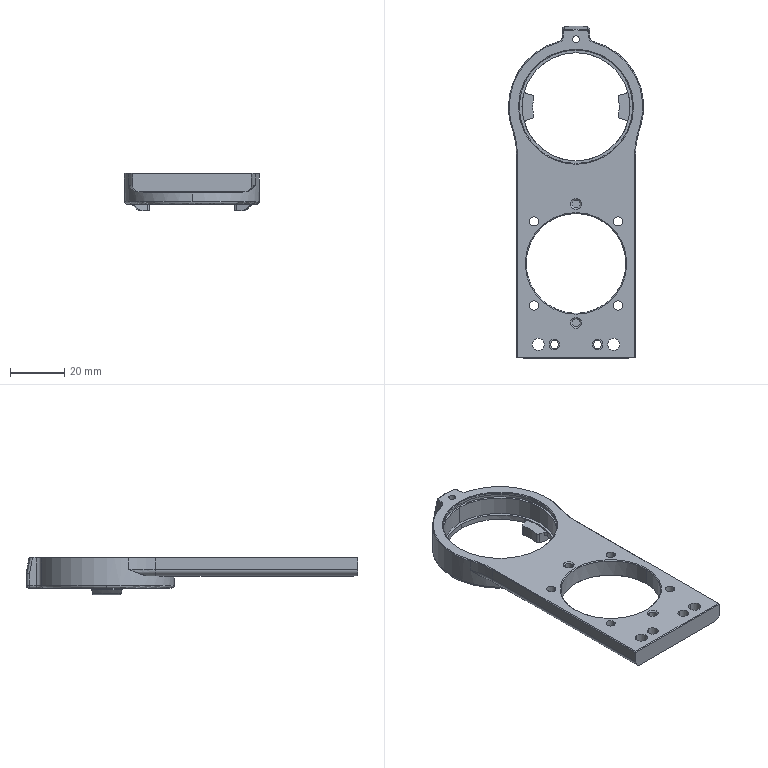NC program | NX | posted with a generic post | part box 50 x 122.9 x 14 mm
Whole program:
N10 G17 G21 G94 G90
(HOLE_MILLING_COPY_COPY_COPY_1 , TOOL : D10JING)
N12 T14 M6
N14 G54
N16 G17 G0 G90 X31.55 Y0. S9500 M3
N18 G43 Z30. H14
N20 Z0.5
N22 G41 G94 G1 X28.392 Y-12.616 F1000. D14
N24 G3 X31.55 Y-16.005 R3.165
N26 X31.55 Y-16.005 Z-0.5 I0. J16.005 F2000.
N28 X31.55 Y-16.005 Z-1.5 I0. J16.005
N30 X31.55 Y-16.005 Z-2.5 I0. J16.005
N32 X31.55 Y-16.005 Z-3.5 I0. J16.005
N34 X31.55 Y-16.005 Z-4.5 I0. J16.005
N36 X31.55 Y-16.005 Z-5.5 I0. J16.005
N38 X31.55 Y-16.005 Z-6.5 I0. J16.005
N40 X31.55 Y-16.005 Z-7.5 I0. J16.005
N42 X31.55 Y-16.005 Z-8.5 I0. J16.005
N44 X31.55 Y-16.005 Z-9.5 I0. J16.005
N46 X34.054 Y-15.808 Z-9.525 R16.005
N48 X47.358 Y2.504 R16.005
N50 X34.054 Y-15.808 R-16.005
N52 X36.642 Y-11.967 R3.165
N54 G40
N56 G1 X31.55 Y0.
N58 G0 Z30.
N60 M5
N62 M2